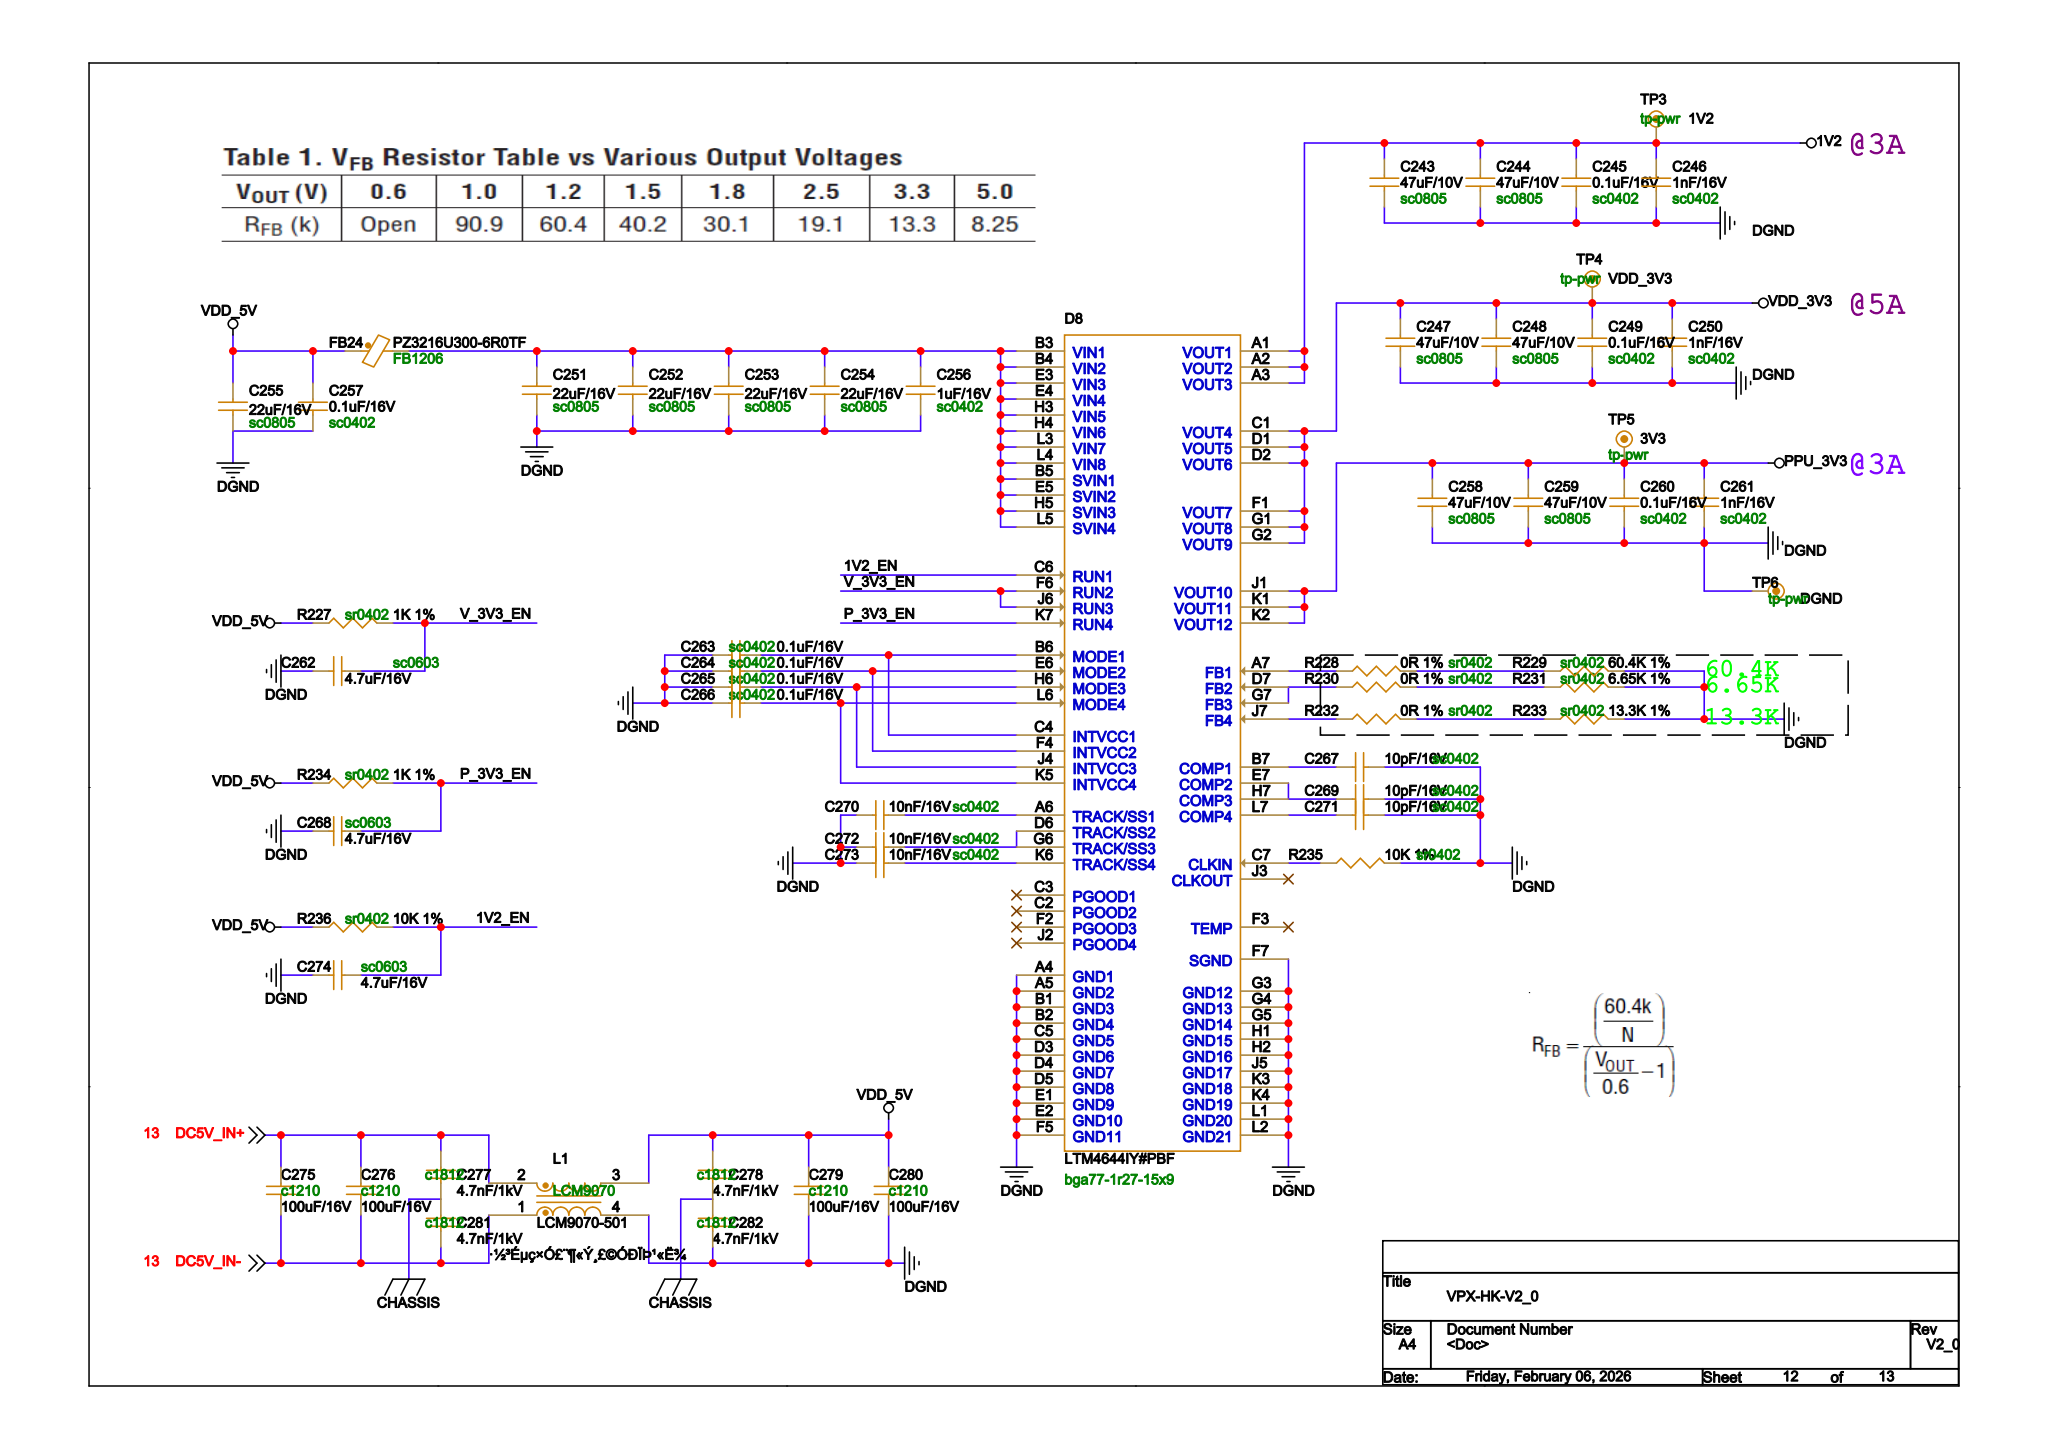Circuit board | Cadence Allegro | 598 parts | 541 nets | one sheet of the schematic
Parts on this sheet (reference | value | footprint):
C243 | 47uF/10V | SC0805
C244 | 47uF/10V | SC0805
C245 | 0.1uF/16V | SC0402
C246 | 1nF/16V | SC0402
C247 | 47uF/10V | SC0805
C248 | 47uF/10V | SC0805
C249 | 0.1uF/16V | SC0402
C250 | 1nF/16V | SC0402
C251 | 22uF/16V | SC0805
C252 | 22uF/16V | SC0805
C253 | 22uF/16V | SC0805
C254 | 22uF/16V | SC0805
C255 | 22uF/16V | SC0805
C256 | 1uF/16V | SC0402
C257 | 0.1uF/16V | SC0402
C258 | 47uF/10V | SC0805
C259 | 47uF/10V | SC0805
C260 | 0.1uF/16V | SC0402
C261 | 1nF/16V | SC0402
C262 | 4.7uF/16V | SC0603
C263 | 0.1uF/16V | SC0402
C264 | 0.1uF/16V | SC0402
C265 | 0.1uF/16V | SC0402
C266 | 0.1uF/16V | SC0402
C267 | 10pF/16V | SC0402
C268 | 4.7uF/16V | SC0603
C269 | 10pF/16V | SC0402
C270 | 10nF/16V | SC0402
C271 | 10pF/16V | SC0402
C272 | 10nF/16V | SC0402
C273 | 10nF/16V | SC0402
C274 | 4.7uF/16V | SC0603
C275 | 100uF/16V | C1210
C276 | 100uF/16V | C1210
C277 | 4.7nF/1kV | C1812
C278 | 4.7nF/1kV | C1812
C279 | 100uF/16V | C1210
C280 | 100uF/16V | C1210
C281 | 4.7nF/1kV | C1812
C282 | 4.7nF/1kV | C1812
D8 | LTM4644IY#PBF | BGA77-1R27-15X9
FB24 | PZ3216U300-6R0TF | FB1206
L1 | LCM9070-501 | LCM9070
R227 | 1K 1% | SR0402
R228 | 0R 1% | SR0402
R229 | 60.4K 1% | SR0402
R230 | 0R 1% | SR0402
R231 | 6.65K 1% | SR0402
R232 | 0R 1% | SR0402
R233 | 13.3K 1% | SR0402
R234 | 1K 1% | SR0402
R235 | 10K 1% | SR0402
R236 | 10K 1% | SR0402
TP3 | PPU_1V2 | TP-PWR
TP4 | VDD_3V3 | TP-PWR
TP5 | PPU_3V3 | TP-PWR
TP6 | PPU_3V3 | TP-PWR
Nets of these parts (net: part-pin ...):
1V2: C243-1 C244-1 C245-1 C246-1 TP3-1 D8-A1 D8-A2 D8-A3
PPU_3V3: C258-1 C259-1 C260-1 C261-1 TP5-1 D8-J1 D8-K1 D8-K2
V_3V3_EN: C262-1 R227-2 D8-F6 D8-J6
DGND: C243-2 C244-2 C245-2 C246-2 C247-2 C248-2 C249-2 C250-2 C251-2 C252-2 C253-2 C254-2 C255-2 C256-2 C257-2 C258-2 C259-2 C260-2 C261-2 C262-2 C263-1 C264-1 C265-1 C266-1 C267-2 C268-2 C269-2 C270-1 C271-2 C272-1 C273-1 C274-2 C279-2 C280-2 C282-2 L1-4 R229-2 R231-2 R233-2 R235-2 TP6-1 D8-A4 D8-A5 D8-B1 D8-B2 D8-C5 D8-D3 D8-D4 D8-D5 D8-E1 D8-E2 D8-F5 D8-F7 D8-G3 D8-G4 D8-G5 D8-H1 D8-H2 D8-J5 D8-K3 D8-K4 D8-L1 D8-L2
P_3V3_EN: C268-1 R234-2 D8-K7
1V2_EN: C274-1 R236-2 D8-C6
DC5V_IN+: C275-1 C276-1 C277-1 L1-2
DC5V_IN-: C275-2 C276-2 C281-2 L1-1
VDD_5V: C255-1 C257-1 C278-1 C279-1 C280-1 FB24-1 L1-3 R227-1 R234-1 R236-1
CHASSIS: C277-2 C278-2 C281-1 C282-1
N32605179: C251-1 C252-1 C253-1 C254-1 C256-1 FB24-2 D8-B3 D8-B4 D8-B5 D8-E3 D8-E4 D8-E5 D8-H3 D8-H4 D8-H5 D8-L3 D8-L4 D8-L5
VDD_3V3: C247-1 C248-1 C249-1 C250-1 TP4-1 D8-C1 D8-D1 D8-D2 D8-F1 D8-G1 D8-G2
N32605647: C266-2 D8-K5 D8-L6
N32605643: C265-2 D8-H6 D8-J4
N32605635: C263-2 D8-B6 D8-C4
N32605633: C264-2 D8-E6 D8-F4
N32605628: R230-2 R231-1
N32605839: R232-2 R233-1
N32605949: C271-1 D8-L7
N32605609: C267-1 D8-B7
N32605144: C269-1 D8-E7 D8-H7
N32605975: C272-2 D8-D6 D8-G6
N32606003: C273-2 D8-K6
N32605149: C270-2 D8-A6
N32605963: R235-1 D8-C7
N32606045: R228-1 D8-A7
N32605626: R230-1 D8-D7 D8-G7
N32605837: R232-1 D8-J7
N32605596: R228-2 R229-1